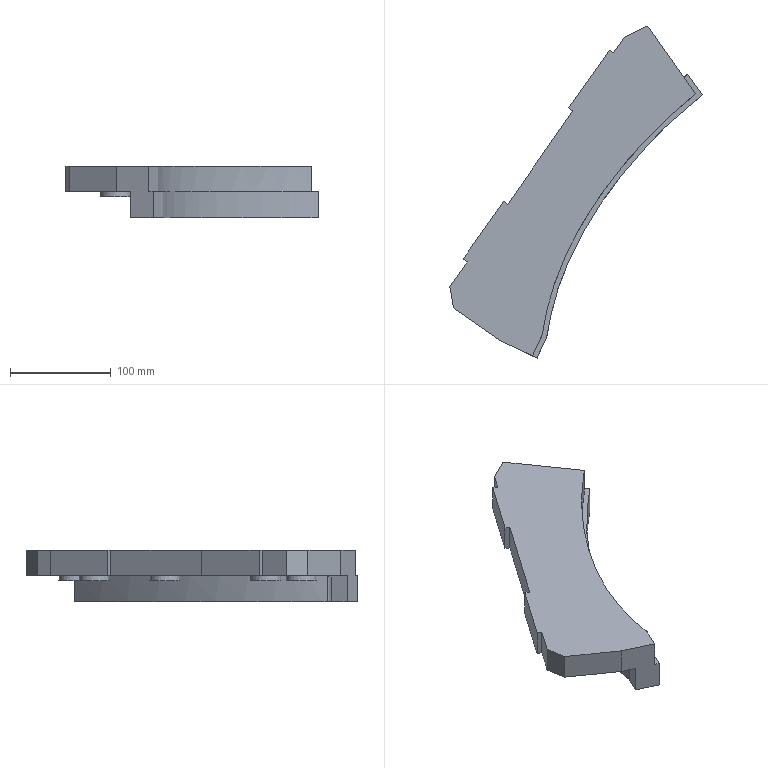Part | NX | features solid 2 | 1 solid | 32 faces | box 249.989 x 328.717 x 51 mm | volume 896333 mm3 | plane 24 | cylinder 5 | spline 3 | commonest cylinder face diameters 30 x5
STEP:
#1=CARTESIAN_POINT('',(-648.758,403.076,20.));
#2=VERTEX_POINT('',#1);
#3=CARTESIAN_POINT('',(-648.758,403.076,45.));
#4=VERTEX_POINT('',#3);
#5=CARTESIAN_POINT('',(-648.758,403.076,70.));
#6=DIRECTION('',(0.,0.,1.));
#7=VECTOR('',#6,1000.);
#8=LINE('',#5,#7);
#9=EDGE_CURVE('',#2,#4,#8,.T.);
#10=ORIENTED_EDGE('',*,*,#9,.F.);
#11=CARTESIAN_POINT('',(-672.097,391.693,20.));
#12=VERTEX_POINT('',#11);
#13=CARTESIAN_POINT('',(-659.778,397.701,20.));
#14=DIRECTION('',(-0.8988,-0.4384,0.));
#15=VECTOR('',#14,1000.);
#16=LINE('',#13,#15);
#17=EDGE_CURVE('',#12,#2,#16,.F.);
#18=ORIENTED_EDGE('',*,*,#17,.F.);
#19=CARTESIAN_POINT('',(-672.097,391.693,45.));
#20=VERTEX_POINT('',#19);
#21=CARTESIAN_POINT('',(-672.097,391.693,70.));
#22=DIRECTION('',(0.,0.,1.));
#23=VECTOR('',#22,1000.);
#24=LINE('',#21,#23);
#25=EDGE_CURVE('',#12,#20,#24,.T.);
#26=ORIENTED_EDGE('',*,*,#25,.T.);
#27=CARTESIAN_POINT('',(-659.778,397.701,45.));
#28=DIRECTION('',(0.8988,0.4384,0.));
#29=VECTOR('',#28,1000.);
#30=LINE('',#27,#29);
#31=EDGE_CURVE('',#20,#4,#30,.T.);
#32=ORIENTED_EDGE('',*,*,#31,.T.);
#33=EDGE_LOOP('',(#10,#18,#26,#32));
#34=FACE_BOUND('',#33,.T.);
#35=CARTESIAN_POINT('',(-659.778,397.701,70.));
#36=DIRECTION('',(-0.4384,0.8988,0.));
#37=DIRECTION('',(-0.8988,-0.4384,0.));
#38=AXIS2_PLACEMENT_3D('',#35,#36,#37);
#39=PLANE('',#38);
#40=ADVANCED_FACE('',(#34),#39,.T.);
#41=CARTESIAN_POINT('',(-758.462,74.359,20.));
#42=VERTEX_POINT('',#41);
#43=CARTESIAN_POINT('',(-595.,335.019,20.));
#44=VERTEX_POINT('',#43);
#45=CARTESIAN_POINT('',(-595.,335.019,20.));
#46=CARTESIAN_POINT('',(-605.153,326.905,20.));
#47=CARTESIAN_POINT('',(-620.012,314.117,20.));
#48=CARTESIAN_POINT('',(-638.944,295.82,20.));
#49=CARTESIAN_POINT('',(-657.041,276.924,20.));
#50=CARTESIAN_POINT('',(-678.202,252.077,20.));
#51=CARTESIAN_POINT('',(-697.186,225.493,20.));
#52=CARTESIAN_POINT('',(-710.926,202.978,20.));
#53=CARTESIAN_POINT('',(-720.284,185.624,20.));
#54=CARTESIAN_POINT('',(-728.613,167.785,20.));
#55=CARTESIAN_POINT('',(-735.843,149.369,20.));
#56=CARTESIAN_POINT('',(-740.793,133.659,20.));
#57=CARTESIAN_POINT('',(-744.038,120.871,20.));
#58=CARTESIAN_POINT('',(-745.744,112.807,20.));
#59=CARTESIAN_POINT('',(-746.914,106.319,20.));
#60=CARTESIAN_POINT('',(-747.543,102.244,20.));
#61=CARTESIAN_POINT('',(-748.031,98.98,20.));
#62=CARTESIAN_POINT('',(-748.271,96.487,20.));
#63=CARTESIAN_POINT('',(-749.155,94.226,20.));
#64=CARTESIAN_POINT('',(-750.586,91.301,20.));
#65=CARTESIAN_POINT('',(-752.275,87.61,20.));
#66=CARTESIAN_POINT('',(-755.033,81.723,20.));
#67=CARTESIAN_POINT('',(-757.089,77.304,20.));
#68=CARTESIAN_POINT('',(-758.462,74.359,20.));
#69=B_SPLINE_CURVE_WITH_KNOTS('',3,(#45,#46,#47,#48,#49,#50,#51,#52,#53,#54,#55,#56,#57,#58,#59,#60,#61,#62,#63,#64,#65,#66,#67,#68),.UNSPECIFIED.,.F.,.F.,(4,1,1,1,1,1,1,1,1,1,1,1,1,1,1,1,1,1,1,1,1,4),(1.053,1.092,1.112,1.131,1.17,1.209,1.228,1.248,1.267,1.287,1.306,1.316,1.326,1.33,1.335,1.338,1.34,1.343,1.345,1.35,1.355,1.364),.UNSPECIFIED.);
#70=EDGE_CURVE('',#42,#44,#69,.F.);
#71=ORIENTED_EDGE('',*,*,#70,.T.);
#72=CARTESIAN_POINT('',(-609.367,355.537,20.));
#73=VERTEX_POINT('',#72);
#74=CARTESIAN_POINT('',(-595.62,335.904,20.));
#75=DIRECTION('',(-0.5736,0.8192,0.));
#76=VECTOR('',#75,1000.);
#77=LINE('',#74,#76);
#78=EDGE_CURVE('',#73,#44,#77,.F.);
#79=ORIENTED_EDGE('',*,*,#78,.F.);
#80=CARTESIAN_POINT('',(-613.276,352.402,20.));
#81=VERTEX_POINT('',#80);
#82=CARTESIAN_POINT('',(-613.276,352.402,20.));
#83=CARTESIAN_POINT('',(-611.977,353.453,20.));
#84=CARTESIAN_POINT('',(-610.674,354.498,20.));
#85=CARTESIAN_POINT('',(-609.367,355.537,20.));
#86=B_SPLINE_CURVE_WITH_KNOTS('',3,(#82,#83,#84,#85),.UNSPECIFIED.,.F.,.F.,(4,4),(0.8753,0.8887),.UNSPECIFIED.);
#87=EDGE_CURVE('',#81,#73,#86,.T.);
#88=ORIENTED_EDGE('',*,*,#87,.F.);
#89=CARTESIAN_POINT('',(-601.776,335.978,20.));
#90=VERTEX_POINT('',#89);
#91=CARTESIAN_POINT('',(-601.969,336.255,20.));
#92=DIRECTION('',(0.5736,-0.8192,0.));
#93=VECTOR('',#92,1000.);
#94=LINE('',#91,#93);
#95=EDGE_CURVE('',#90,#81,#94,.F.);
#96=ORIENTED_EDGE('',*,*,#95,.F.);
#97=CARTESIAN_POINT('',(-762.994,76.472,20.));
#98=VERTEX_POINT('',#97);
#99=CARTESIAN_POINT('',(-601.776,335.978,20.));
#100=CARTESIAN_POINT('',(-611.865,327.771,20.));
#101=CARTESIAN_POINT('',(-631.456,310.599,20.));
#102=CARTESIAN_POINT('',(-658.632,282.914,20.));
#103=CARTESIAN_POINT('',(-683.631,253.231,20.));
#104=CARTESIAN_POINT('',(-702.468,226.555,20.));
#105=CARTESIAN_POINT('',(-715.855,204.414,20.));
#106=CARTESIAN_POINT('',(-725.004,187.347,20.));
#107=CARTESIAN_POINT('',(-733.184,169.786,20.));
#108=CARTESIAN_POINT('',(-740.313,151.694,20.));
#109=CARTESIAN_POINT('',(-745.285,136.104,20.));
#110=CARTESIAN_POINT('',(-748.577,123.395,20.));
#111=CARTESIAN_POINT('',(-750.336,115.344,20.));
#112=CARTESIAN_POINT('',(-751.55,108.834,20.));
#113=CARTESIAN_POINT('',(-752.231,104.739,20.));
#114=CARTESIAN_POINT('',(-752.713,101.439,20.));
#115=CARTESIAN_POINT('',(-753.022,99.38,20.));
#116=CARTESIAN_POINT('',(-753.186,97.703,20.));
#117=CARTESIAN_POINT('',(-753.603,96.55,20.));
#118=CARTESIAN_POINT('',(-754.149,95.443,20.));
#119=CARTESIAN_POINT('',(-754.839,93.954,20.));
#120=CARTESIAN_POINT('',(-755.709,92.095,20.));
#121=CARTESIAN_POINT('',(-757.096,89.119,20.));
#122=CARTESIAN_POINT('',(-758.831,85.399,20.));
#123=CARTESIAN_POINT('',(-760.912,80.936,20.));
#124=CARTESIAN_POINT('',(-762.3,77.96,20.));
#125=CARTESIAN_POINT('',(-762.994,76.472,20.));
#126=B_SPLINE_CURVE_WITH_KNOTS('',3,(#99,#100,#101,#102,#103,#104,#105,#106,#107,#108,#109,#110,#111,#112,#113,#114,#115,#116,#117,#118,#119,#120,#121,#122,#123,#124,#125),.UNSPECIFIED.,.F.,.F.,(4,1,1,1,1,1,1,1,1,1,1,1,1,1,1,1,1,1,1,1,1,1,1,1,4),(0.8327,0.8717,0.9106,0.9496,0.9886,1.008,1.028,1.047,1.066,1.086,1.096,1.105,1.11,1.115,1.118,1.12,1.121,1.122,1.124,1.125,1.127,1.13,1.135,1.14,1.144),.UNSPECIFIED.);
#127=EDGE_CURVE('',#98,#90,#126,.F.);
#128=ORIENTED_EDGE('',*,*,#127,.F.);
#129=CARTESIAN_POINT('',(-758.462,74.359,20.));
#130=DIRECTION('',(-0.9063,0.4226,0.));
#131=VECTOR('',#130,1000.);
#132=LINE('',#129,#131);
#133=EDGE_CURVE('',#98,#42,#132,.F.);
#134=ORIENTED_EDGE('',*,*,#133,.T.);
#135=EDGE_LOOP('',(#71,#79,#88,#96,#128,#134));
#136=FACE_BOUND('',#135,.T.);
#137=CARTESIAN_POINT('',(-561.977,359.461,20.));
#138=DIRECTION('',(0.,0.,1.));
#139=DIRECTION('',(1.,0.,0.));
#140=AXIS2_PLACEMENT_3D('',#137,#138,#139);
#141=PLANE('',#140);
#142=ADVANCED_FACE('',(#136),#141,.T.);
#143=CARTESIAN_POINT('',(-595.,335.019,-6.));
#144=VERTEX_POINT('',#143);
#145=CARTESIAN_POINT('',(-595.,335.019,7.));
#146=DIRECTION('',(0.,0.,-1.));
#147=VECTOR('',#146,1000.);
#148=LINE('',#145,#147);
#149=EDGE_CURVE('',#44,#144,#148,.T.);
#150=ORIENTED_EDGE('',*,*,#149,.F.);
#151=ORIENTED_EDGE('',*,*,#70,.F.);
#152=CARTESIAN_POINT('',(-758.462,74.359,-6.));
#153=VERTEX_POINT('',#152);
#154=CARTESIAN_POINT('',(-758.462,74.359,70.));
#155=DIRECTION('',(0.,0.,-1.));
#156=VECTOR('',#155,1000.);
#157=LINE('',#154,#156);
#158=EDGE_CURVE('',#42,#153,#157,.T.);
#159=ORIENTED_EDGE('',*,*,#158,.T.);
#160=CARTESIAN_POINT('',(-595.,335.019,-6.));
#161=CARTESIAN_POINT('',(-605.196,326.871,-6.));
#162=CARTESIAN_POINT('',(-625.159,309.672,-6.));
#163=CARTESIAN_POINT('',(-652.791,281.906,-6.));
#164=CARTESIAN_POINT('',(-678.136,252.163,-6.));
#165=CARTESIAN_POINT('',(-697.173,225.515,-6.));
#166=CARTESIAN_POINT('',(-710.901,203.021,-6.));
#167=CARTESIAN_POINT('',(-720.24,185.709,-6.));
#168=CARTESIAN_POINT('',(-728.575,167.875,-6.));
#169=CARTESIAN_POINT('',(-735.812,149.456,-6.));
#170=CARTESIAN_POINT('',(-740.761,133.769,-6.));
#171=CARTESIAN_POINT('',(-744.012,120.984,-6.));
#172=CARTESIAN_POINT('',(-745.72,112.928,-6.));
#173=CARTESIAN_POINT('',(-746.895,106.436,-6.));
#174=CARTESIAN_POINT('',(-747.528,102.339,-6.));
#175=CARTESIAN_POINT('',(-748.022,99.056,-6.));
#176=CARTESIAN_POINT('',(-748.26,96.545,-6.));
#177=CARTESIAN_POINT('',(-749.131,94.27,-6.));
#178=CARTESIAN_POINT('',(-750.569,91.341,-6.));
#179=CARTESIAN_POINT('',(-752.26,87.64,-6.));
#180=CARTESIAN_POINT('',(-754.334,83.216,-6.));
#181=CARTESIAN_POINT('',(-756.397,78.787,-6.));
#182=CARTESIAN_POINT('',(-757.774,75.835,-6.));
#183=CARTESIAN_POINT('',(-758.462,74.359,-6.));
#184=B_SPLINE_CURVE_WITH_KNOTS('',3,(#160,#161,#162,#163,#164,#165,#166,#167,#168,#169,#170,#171,#172,#173,#174,#175,#176,#177,#178,#179,#180,#181,#182,#183),.UNSPECIFIED.,.F.,.F.,(4,1,1,1,1,1,1,1,1,1,1,1,1,1,1,1,1,1,1,1,1,4),(1.071,1.11,1.149,1.188,1.227,1.246,1.266,1.285,1.305,1.324,1.334,1.344,1.348,1.353,1.356,1.358,1.361,1.363,1.368,1.373,1.378,1.382),.UNSPECIFIED.);
#185=EDGE_CURVE('',#153,#144,#184,.F.);
#186=ORIENTED_EDGE('',*,*,#185,.T.);
#187=EDGE_LOOP('',(#150,#151,#159,#186));
#188=FACE_BOUND('',#187,.T.);
#189=CARTESIAN_POINT('',(-758.462,74.359,20.));
#190=CARTESIAN_POINT('',(-758.462,74.359,-6.));
#191=CARTESIAN_POINT('',(-757.77,75.844,20.));
#192=CARTESIAN_POINT('',(-757.77,75.844,-6.));
#193=CARTESIAN_POINT('',(-756.384,78.814,20.));
#194=CARTESIAN_POINT('',(-756.384,78.814,-6.));
#195=CARTESIAN_POINT('',(-754.31,83.27,20.));
#196=CARTESIAN_POINT('',(-754.31,83.27,-6.));
#197=CARTESIAN_POINT('',(-752.221,87.72,20.));
#198=CARTESIAN_POINT('',(-752.221,87.72,-6.));
#199=CARTESIAN_POINT('',(-750.525,91.449,20.));
#200=CARTESIAN_POINT('',(-750.525,91.449,-6.));
#201=CARTESIAN_POINT('',(-749.067,94.385,20.));
#202=CARTESIAN_POINT('',(-749.067,94.385,-6.));
#203=CARTESIAN_POINT('',(-748.233,96.708,20.));
#204=CARTESIAN_POINT('',(-748.233,96.708,-6.));
#205=CARTESIAN_POINT('',(-748.008,99.169,20.));
#206=CARTESIAN_POINT('',(-748.008,99.169,-6.));
#207=CARTESIAN_POINT('',(-747.517,102.405,20.));
#208=CARTESIAN_POINT('',(-747.517,102.405,-6.));
#209=CARTESIAN_POINT('',(-746.892,106.453,20.));
#210=CARTESIAN_POINT('',(-746.892,106.453,-6.));
#211=CARTESIAN_POINT('',(-745.725,112.898,20.));
#212=CARTESIAN_POINT('',(-745.725,112.898,-6.));
#213=CARTESIAN_POINT('',(-744.029,120.909,20.));
#214=CARTESIAN_POINT('',(-744.029,120.909,-6.));
#215=CARTESIAN_POINT('',(-740.804,133.612,20.));
#216=CARTESIAN_POINT('',(-740.804,133.612,-6.));
#217=CARTESIAN_POINT('',(-735.88,149.258,20.));
#218=CARTESIAN_POINT('',(-735.88,149.258,-6.));
#219=CARTESIAN_POINT('',(-728.697,167.587,20.));
#220=CARTESIAN_POINT('',(-728.697,167.587,-6.));
#221=CARTESIAN_POINT('',(-720.391,185.411,20.));
#222=CARTESIAN_POINT('',(-720.391,185.411,-6.));
#223=CARTESIAN_POINT('',(-711.068,202.728,20.));
#224=CARTESIAN_POINT('',(-711.068,202.728,-6.));
#225=CARTESIAN_POINT('',(-697.423,225.135,20.));
#226=CARTESIAN_POINT('',(-697.423,225.135,-6.));
#227=CARTESIAN_POINT('',(-678.389,251.849,20.));
#228=CARTESIAN_POINT('',(-678.389,251.849,-6.));
#229=CARTESIAN_POINT('',(-644.374,291.818,20.));
#230=CARTESIAN_POINT('',(-644.374,291.818,-6.));
#231=CARTESIAN_POINT('',(-615.478,318.655,20.));
#232=CARTESIAN_POINT('',(-615.478,318.655,-6.));
#233=CARTESIAN_POINT('',(-595.,335.019,20.));
#234=CARTESIAN_POINT('',(-595.,335.019,-6.));
#235=B_SPLINE_SURFACE_WITH_KNOTS('',3,1,((#189,#190),(#191,#192),(#193,#194),(#195,#196),(#197,#198),(#199,#200),(#201,#202),(#203,#204),(#205,#206),(#207,#208),(#209,#210),(#211,#212),(#213,#214),(#215,#216),(#217,#218),(#219,#220),(#221,#222),(#223,#224),(#225,#226),(#227,#228),(#229,#230),(#231,#232),(#233,#234)),.SURF_OF_LINEAR_EXTRUSION.,.F.,.F.,.F.,(4,1,1,1,1,1,1,1,1,1,1,1,1,1,1,1,1,1,1,1,4),(2,2),(0.003106,0.007303,0.0115,0.01569,0.01989,0.02199,0.02409,0.02619,0.02828,0.03248,0.03668,0.04507,0.05346,0.07025,0.08703,0.1038,0.1206,0.1374,0.171,0.2045,0.2717),(0.,1.),.UNSPECIFIED.);
#236=ADVANCED_FACE('',(#188),#235,.F.);
#237=CARTESIAN_POINT('',(-609.367,355.537,-6.));
#238=VERTEX_POINT('',#237);
#239=CARTESIAN_POINT('',(105.312,-665.13,-6.));
#240=DIRECTION('',(-0.5736,0.8192,0.));
#241=VECTOR('',#240,1000.);
#242=LINE('',#239,#241);
#243=EDGE_CURVE('',#144,#238,#242,.T.);
#244=ORIENTED_EDGE('',*,*,#243,.F.);
#245=ORIENTED_EDGE('',*,*,#185,.F.);
#246=CARTESIAN_POINT('',(-781.12,84.924,-6.));
#247=VERTEX_POINT('',#246);
#248=CARTESIAN_POINT('',(-2805.507,1028.912,-6.));
#249=DIRECTION('',(0.9063,-0.4226,0.));
#250=VECTOR('',#249,1000.);
#251=LINE('',#248,#250);
#252=EDGE_CURVE('',#247,#153,#251,.T.);
#253=ORIENTED_EDGE('',*,*,#252,.F.);
#254=CARTESIAN_POINT('',(-609.367,355.537,-6.));
#255=CARTESIAN_POINT('',(-630.504,338.743,-6.));
#256=CARTESIAN_POINT('',(-670.028,302.396,-6.));
#257=CARTESIAN_POINT('',(-712.936,248.72,-6.));
#258=CARTESIAN_POINT('',(-740.771,201.703,-6.));
#259=CARTESIAN_POINT('',(-754.778,170.697,-6.));
#260=CARTESIAN_POINT('',(-763.749,144.683,-6.));
#261=CARTESIAN_POINT('',(-768.036,127.873,-6.));
#262=CARTESIAN_POINT('',(-771.159,114.324,-6.));
#263=CARTESIAN_POINT('',(-771.858,103.55,-6.));
#264=CARTESIAN_POINT('',(-776.875,94.381,-6.));
#265=CARTESIAN_POINT('',(-779.658,88.059,-6.));
#266=CARTESIAN_POINT('',(-781.12,84.924,-6.));
#267=B_SPLINE_CURVE_WITH_KNOTS('',3,(#254,#255,#256,#257,#258,#259,#260,#261,#262,#263,#264,#265,#266),.UNSPECIFIED.,.F.,.F.,(4,1,1,1,1,1,1,1,1,1,4),(0.205,0.2866,0.3682,0.409,0.4498,0.4702,0.4906,0.5008,0.511,0.5212,0.5314),.UNSPECIFIED.);
#268=EDGE_CURVE('',#247,#238,#267,.F.);
#269=ORIENTED_EDGE('',*,*,#268,.T.);
#270=EDGE_LOOP('',(#244,#245,#253,#269));
#271=FACE_BOUND('',#270,.T.);
#272=CARTESIAN_POINT('',(-80.139,-794.984,-6.));
#273=DIRECTION('',(0.,0.,1.));
#274=DIRECTION('',(1.,0.,0.));
#275=AXIS2_PLACEMENT_3D('',#272,#273,#274);
#276=PLANE('',#275);
#277=ADVANCED_FACE('',(#271),#276,.F.);
#278=CARTESIAN_POINT('',(-601.776,335.978,45.));
#279=VERTEX_POINT('',#278);
#280=CARTESIAN_POINT('',(-601.969,336.255,45.));
#281=DIRECTION('',(-0.5736,0.8192,0.));
#282=VECTOR('',#281,1000.);
#283=LINE('',#280,#282);
#284=EDGE_CURVE('',#279,#4,#283,.T.);
#285=ORIENTED_EDGE('',*,*,#284,.T.);
#286=ORIENTED_EDGE('',*,*,#31,.F.);
#287=CARTESIAN_POINT('',(-682.817,376.384,45.));
#288=VERTEX_POINT('',#287);
#289=CARTESIAN_POINT('',(-902.294,62.938,45.));
#290=DIRECTION('',(0.5736,0.8192,0.));
#291=VECTOR('',#290,1000.);
#292=LINE('',#289,#291);
#293=EDGE_CURVE('',#288,#20,#292,.T.);
#294=ORIENTED_EDGE('',*,*,#293,.F.);
#295=CARTESIAN_POINT('',(-686.912,379.252,45.));
#296=VERTEX_POINT('',#295);
#297=CARTESIAN_POINT('',(271.949,-292.15,45.));
#298=DIRECTION('',(-0.8192,0.5736,0.));
#299=VECTOR('',#298,1000.);
#300=LINE('',#297,#299);
#301=EDGE_CURVE('',#288,#296,#300,.T.);
#302=ORIENTED_EDGE('',*,*,#301,.T.);
#303=CARTESIAN_POINT('',(-727.063,321.911,45.));
#304=VERTEX_POINT('',#303);
#305=CARTESIAN_POINT('',(-675.441,395.635,45.));
#306=DIRECTION('',(0.5736,0.8192,0.));
#307=VECTOR('',#306,1000.);
#308=LINE('',#305,#307);
#309=EDGE_CURVE('',#304,#296,#308,.T.);
#310=ORIENTED_EDGE('',*,*,#309,.F.);
#311=CARTESIAN_POINT('',(-722.967,319.043,45.));
#312=VERTEX_POINT('',#311);
#313=CARTESIAN_POINT('',(231.799,-349.491,45.));
#314=DIRECTION('',(-0.8192,0.5736,0.));
#315=VECTOR('',#314,1000.);
#316=LINE('',#313,#315);
#317=EDGE_CURVE('',#312,#304,#316,.T.);
#318=ORIENTED_EDGE('',*,*,#317,.F.);
#319=CARTESIAN_POINT('',(-787.631,226.693,45.));
#320=VERTEX_POINT('',#319);
#321=CARTESIAN_POINT('',(-902.294,62.938,45.));
#322=DIRECTION('',(0.5736,0.8192,0.));
#323=VECTOR('',#322,1000.);
#324=LINE('',#321,#323);
#325=EDGE_CURVE('',#320,#312,#324,.T.);
#326=ORIENTED_EDGE('',*,*,#325,.F.);
#327=CARTESIAN_POINT('',(-791.727,229.561,45.));
#328=VERTEX_POINT('',#327);
#329=CARTESIAN_POINT('',(167.134,-441.841,45.));
#330=DIRECTION('',(-0.8192,0.5736,0.));
#331=VECTOR('',#330,1000.);
#332=LINE('',#329,#331);
#333=EDGE_CURVE('',#320,#328,#332,.T.);
#334=ORIENTED_EDGE('',*,*,#333,.T.);
#335=CARTESIAN_POINT('',(-831.877,172.22,45.));
#336=VERTEX_POINT('',#335);
#337=CARTESIAN_POINT('',(-846.217,151.741,45.));
#338=DIRECTION('',(0.5736,0.8192,0.));
#339=VECTOR('',#338,1000.);
#340=LINE('',#337,#339);
#341=EDGE_CURVE('',#336,#328,#340,.T.);
#342=ORIENTED_EDGE('',*,*,#341,.F.);
#343=CARTESIAN_POINT('',(-827.782,169.352,45.));
#344=VERTEX_POINT('',#343);
#345=CARTESIAN_POINT('',(126.984,-499.182,45.));
#346=DIRECTION('',(-0.8192,0.5736,0.));
#347=VECTOR('',#346,1000.);
#348=LINE('',#345,#347);
#349=EDGE_CURVE('',#344,#336,#348,.T.);
#350=ORIENTED_EDGE('',*,*,#349,.F.);
#351=CARTESIAN_POINT('',(-844.989,144.778,45.));
#352=VERTEX_POINT('',#351);
#353=CARTESIAN_POINT('',(-902.294,62.938,45.));
#354=DIRECTION('',(0.5736,0.8192,0.));
#355=VECTOR('',#354,1000.);
#356=LINE('',#353,#355);
#357=EDGE_CURVE('',#352,#344,#356,.T.);
#358=ORIENTED_EDGE('',*,*,#357,.F.);
#359=CARTESIAN_POINT('',(-841.305,123.887,45.));
#360=VERTEX_POINT('',#359);
#361=CARTESIAN_POINT('',(-799.958,-110.607,45.));
#362=DIRECTION('',(-0.1736,0.9848,0.));
#363=VECTOR('',#362,1000.);
#364=LINE('',#361,#363);
#365=EDGE_CURVE('',#352,#360,#364,.F.);
#366=ORIENTED_EDGE('',*,*,#365,.T.);
#367=CARTESIAN_POINT('',(-794.714,91.264,45.));
#368=VERTEX_POINT('',#367);
#369=CARTESIAN_POINT('',(-875.296,147.687,45.));
#370=DIRECTION('',(-0.8192,0.5736,0.));
#371=VECTOR('',#370,1000.);
#372=LINE('',#369,#371);
#373=EDGE_CURVE('',#360,#368,#372,.F.);
#374=ORIENTED_EDGE('',*,*,#373,.T.);
#375=CARTESIAN_POINT('',(-762.994,76.472,45.));
#376=VERTEX_POINT('',#375);
#377=CARTESIAN_POINT('',(-2805.507,1028.912,45.));
#378=DIRECTION('',(0.9063,-0.4226,0.));
#379=VECTOR('',#378,1000.);
#380=LINE('',#377,#379);
#381=EDGE_CURVE('',#368,#376,#380,.T.);
#382=ORIENTED_EDGE('',*,*,#381,.T.);
#383=CARTESIAN_POINT('',(-762.994,76.472,45.));
#384=CARTESIAN_POINT('',(-762.296,77.969,45.));
#385=CARTESIAN_POINT('',(-760.899,80.963,45.));
#386=CARTESIAN_POINT('',(-758.805,85.454,45.));
#387=CARTESIAN_POINT('',(-757.06,89.196,45.));
#388=CARTESIAN_POINT('',(-755.665,92.19,45.));
#389=CARTESIAN_POINT('',(-754.789,94.061,45.));
#390=CARTESIAN_POINT('',(-754.096,95.559,45.));
#391=CARTESIAN_POINT('',(-753.541,96.672,45.));
#392=CARTESIAN_POINT('',(-753.168,97.842,45.));
#393=CARTESIAN_POINT('',(-753.006,99.505,45.));
#394=CARTESIAN_POINT('',(-752.696,101.551,45.));
#395=CARTESIAN_POINT('',(-752.217,104.829,45.));
#396=CARTESIAN_POINT('',(-751.537,108.902,45.));
#397=CARTESIAN_POINT('',(-750.329,115.381,45.));
#398=CARTESIAN_POINT('',(-748.574,123.409,45.));
#399=CARTESIAN_POINT('',(-745.293,136.072,45.));
#400=CARTESIAN_POINT('',(-740.361,151.552,45.));
#401=CARTESIAN_POINT('',(-733.25,169.635,45.));
#402=CARTESIAN_POINT('',(-725.048,187.263,45.));
#403=CARTESIAN_POINT('',(-715.826,204.474,45.));
#404=CARTESIAN_POINT('',(-702.266,226.868,45.));
#405=CARTESIAN_POINT('',(-683.587,253.27,45.));
#406=CARTESIAN_POINT('',(-658.666,282.876,45.));
#407=CARTESIAN_POINT('',(-631.52,310.539,45.));
#408=CARTESIAN_POINT('',(-611.886,327.754,45.));
#409=CARTESIAN_POINT('',(-601.776,335.978,45.));
#410=B_SPLINE_CURVE_WITH_KNOTS('',3,(#383,#384,#385,#386,#387,#388,#389,#390,#391,#392,#393,#394,#395,#396,#397,#398,#399,#400,#401,#402,#403,#404,#405,#406,#407,#408,#409),.UNSPECIFIED.,.F.,.F.,(4,1,1,1,1,1,1,1,1,1,1,1,1,1,1,1,1,1,1,1,1,1,1,1,4),(0.,0.00491,0.00982,0.01473,0.01718,0.01964,0.02087,0.02209,0.02332,0.02455,0.027,0.02946,0.03437,0.03928,0.0491,0.05892,0.07856,0.0982,0.1178,0.1375,0.1571,0.1964,0.2357,0.2749,0.3142),.UNSPECIFIED.);
#411=EDGE_CURVE('',#376,#279,#410,.T.);
#412=ORIENTED_EDGE('',*,*,#411,.T.);
#413=EDGE_LOOP('',(#285,#286,#294,#302,#310,#318,#326,#334,#342,#350,#358,#366,#374,#382,#412));
#414=FACE_BOUND('',#413,.T.);
#415=CARTESIAN_POINT('',(-80.139,-794.984,45.));
#416=DIRECTION('',(0.,0.,1.));
#417=DIRECTION('',(1.,0.,0.));
#418=AXIS2_PLACEMENT_3D('',#415,#416,#417);
#419=PLANE('',#418);
#420=ADVANCED_FACE('',(#414),#419,.T.);
#421=CARTESIAN_POINT('',(-660.611,355.558,20.));
#422=VERTEX_POINT('',#421);
#423=CARTESIAN_POINT('',(-645.611,355.558,20.));
#424=DIRECTION('',(0.,0.,-1.));
#425=DIRECTION('',(-1.,0.,0.));
#426=AXIS2_PLACEMENT_3D('',#423,#424,#425);
#427=CIRCLE('',#426,15.);
#428=EDGE_CURVE('',#422,#422,#427,.F.);
#429=ORIENTED_EDGE('',*,*,#428,.T.);
#430=EDGE_LOOP('',(#429));
#431=FACE_BOUND('',#430,.T.);
#432=CARTESIAN_POINT('',(-690.611,335.558,20.));
#433=VERTEX_POINT('',#432);
#434=CARTESIAN_POINT('',(-675.611,335.558,20.));
#435=DIRECTION('',(0.,0.,-1.));
#436=DIRECTION('',(-1.,0.,0.));
#437=AXIS2_PLACEMENT_3D('',#434,#435,#436);
#438=CIRCLE('',#437,15.);
#439=EDGE_CURVE('',#433,#433,#438,.F.);
#440=ORIENTED_EDGE('',*,*,#439,.T.);
#441=EDGE_LOOP('',(#440));
#442=FACE_BOUND('',#441,.T.);
#443=CARTESIAN_POINT('',(-810.611,130.558,20.));
#444=VERTEX_POINT('',#443);
#445=CARTESIAN_POINT('',(-795.611,130.558,20.));
#446=DIRECTION('',(0.,0.,-1.));
#447=DIRECTION('',(-1.,0.,0.));
#448=AXIS2_PLACEMENT_3D('',#445,#446,#447);
#449=CIRCLE('',#448,15.);
#450=EDGE_CURVE('',#444,#444,#449,.T.);
#451=ORIENTED_EDGE('',*,*,#450,.F.);
#452=EDGE_LOOP('',(#451));
#453=FACE_BOUND('',#452,.T.);
#454=CARTESIAN_POINT('',(-810.611,165.558,20.));
#455=VERTEX_POINT('',#454);
#456=CARTESIAN_POINT('',(-795.611,165.558,20.));
#457=DIRECTION('',(0.,0.,-1.));
#458=DIRECTION('',(-1.,0.,0.));
#459=AXIS2_PLACEMENT_3D('',#456,#457,#458);
#460=CIRCLE('',#459,15.);
#461=EDGE_CURVE('',#455,#455,#460,.T.);
#462=ORIENTED_EDGE('',*,*,#461,.F.);
#463=EDGE_LOOP('',(#462));
#464=FACE_BOUND('',#463,.T.);
#465=CARTESIAN_POINT('',(-735.611,265.558,20.));
#466=VERTEX_POINT('',#465);
#467=CARTESIAN_POINT('',(-720.611,265.558,20.));
#468=DIRECTION('',(0.,0.,-1.));
#469=DIRECTION('',(-1.,0.,0.));
#470=AXIS2_PLACEMENT_3D('',#467,#468,#469);
#471=CIRCLE('',#470,15.);
#472=EDGE_CURVE('',#466,#466,#471,.T.);
#473=ORIENTED_EDGE('',*,*,#472,.F.);
#474=EDGE_LOOP('',(#473));
#475=FACE_BOUND('',#474,.T.);
#476=ORIENTED_EDGE('',*,*,#17,.T.);
#477=CARTESIAN_POINT('',(-601.969,336.255,20.));
#478=DIRECTION('',(0.5736,-0.8192,0.));
#479=VECTOR('',#478,1000.);
#480=LINE('',#477,#479);
#481=EDGE_CURVE('',#81,#2,#480,.F.);
#482=ORIENTED_EDGE('',*,*,#481,.F.);
#483=CARTESIAN_POINT('',(-781.12,84.924,20.));
#484=VERTEX_POINT('',#483);
#485=CARTESIAN_POINT('',(-613.276,352.402,20.));
#486=CARTESIAN_POINT('',(-633.961,335.665,20.));
#487=CARTESIAN_POINT('',(-672.617,299.523,20.));
#488=CARTESIAN_POINT('',(-714.519,246.391,20.));
#489=CARTESIAN_POINT('',(-741.653,199.957,20.));
#490=CARTESIAN_POINT('',(-755.295,169.366,20.));
#491=CARTESIAN_POINT('',(-764.029,143.734,20.));
#492=CARTESIAN_POINT('',(-768.193,127.17,20.));
#493=CARTESIAN_POINT('',(-771.254,113.831,20.));
#494=CARTESIAN_POINT('',(-771.879,103.202,20.));
#495=CARTESIAN_POINT('',(-776.98,94.242,20.));
#496=CARTESIAN_POINT('',(-779.682,88.009,20.));
#497=CARTESIAN_POINT('',(-781.12,84.924,20.));
#498=B_SPLINE_CURVE_WITH_KNOTS('',3,(#485,#486,#487,#488,#489,#490,#491,#492,#493,#494,#495,#496,#497),.UNSPECIFIED.,.F.,.F.,(4,1,1,1,1,1,1,1,1,1,4),(0.9033,0.9838,1.064,1.105,1.145,1.165,1.185,1.195,1.205,1.215,1.225),.UNSPECIFIED.);
#499=EDGE_CURVE('',#484,#81,#498,.F.);
#500=ORIENTED_EDGE('',*,*,#499,.F.);
#501=CARTESIAN_POINT('',(-794.714,91.264,20.));
#502=VERTEX_POINT('',#501);
#503=CARTESIAN_POINT('',(-2805.507,1028.912,20.));
#504=DIRECTION('',(-0.9063,0.4226,0.));
#505=VECTOR('',#504,1000.);
#506=LINE('',#503,#505);
#507=EDGE_CURVE('',#502,#484,#506,.F.);
#508=ORIENTED_EDGE('',*,*,#507,.F.);
#509=CARTESIAN_POINT('',(-841.305,123.887,20.));
#510=VERTEX_POINT('',#509);
#511=CARTESIAN_POINT('',(-762.446,68.669,20.));
#512=DIRECTION('',(-0.8192,0.5736,0.));
#513=VECTOR('',#512,1000.);
#514=LINE('',#511,#513);
#515=EDGE_CURVE('',#502,#510,#514,.T.);
#516=ORIENTED_EDGE('',*,*,#515,.T.);
#517=CARTESIAN_POINT('',(-844.989,144.778,20.));
#518=VERTEX_POINT('',#517);
#519=CARTESIAN_POINT('',(-841.305,123.887,20.));
#520=DIRECTION('',(-0.1736,0.9848,0.));
#521=VECTOR('',#520,1000.);
#522=LINE('',#519,#521);
#523=EDGE_CURVE('',#510,#518,#522,.T.);
#524=ORIENTED_EDGE('',*,*,#523,.T.);
#525=CARTESIAN_POINT('',(-827.782,169.352,20.));
#526=VERTEX_POINT('',#525);
#527=CARTESIAN_POINT('',(-902.294,62.938,20.));
#528=DIRECTION('',(-0.5736,-0.8192,0.));
#529=VECTOR('',#528,1000.);
#530=LINE('',#527,#529);
#531=EDGE_CURVE('',#518,#526,#530,.F.);
#532=ORIENTED_EDGE('',*,*,#531,.T.);
#533=CARTESIAN_POINT('',(-831.877,172.22,20.));
#534=VERTEX_POINT('',#533);
#535=CARTESIAN_POINT('',(-738.746,107.009,20.));
#536=DIRECTION('',(0.8192,-0.5736,0.));
#537=VECTOR('',#536,1000.);
#538=LINE('',#535,#537);
#539=EDGE_CURVE('',#526,#534,#538,.F.);
#540=ORIENTED_EDGE('',*,*,#539,.T.);
#541=CARTESIAN_POINT('',(-791.727,229.561,20.));
#542=VERTEX_POINT('',#541);
#543=CARTESIAN_POINT('',(-846.217,151.741,20.));
#544=DIRECTION('',(0.5736,0.8192,0.));
#545=VECTOR('',#544,1000.);
#546=LINE('',#543,#545);
#547=EDGE_CURVE('',#534,#542,#546,.T.);
#548=ORIENTED_EDGE('',*,*,#547,.T.);
#549=CARTESIAN_POINT('',(-787.631,226.693,20.));
#550=VERTEX_POINT('',#549);
#551=CARTESIAN_POINT('',(-698.596,164.349,20.));
#552=DIRECTION('',(0.8192,-0.5736,0.));
#553=VECTOR('',#552,1000.);
#554=LINE('',#551,#553);
#555=EDGE_CURVE('',#550,#542,#554,.F.);
#556=ORIENTED_EDGE('',*,*,#555,.F.);
#557=CARTESIAN_POINT('',(-722.967,319.043,20.));
#558=VERTEX_POINT('',#557);
#559=CARTESIAN_POINT('',(-902.294,62.938,20.));
#560=DIRECTION('',(-0.5736,-0.8192,0.));
#561=VECTOR('',#560,1000.);
#562=LINE('',#559,#561);
#563=EDGE_CURVE('',#550,#558,#562,.F.);
#564=ORIENTED_EDGE('',*,*,#563,.T.);
#565=CARTESIAN_POINT('',(-727.063,321.911,20.));
#566=VERTEX_POINT('',#565);
#567=CARTESIAN_POINT('',(-633.931,256.7,20.));
#568=DIRECTION('',(0.8192,-0.5736,0.));
#569=VECTOR('',#568,1000.);
#570=LINE('',#567,#569);
#571=EDGE_CURVE('',#558,#566,#570,.F.);
#572=ORIENTED_EDGE('',*,*,#571,.T.);
#573=CARTESIAN_POINT('',(-686.912,379.252,20.));
#574=VERTEX_POINT('',#573);
#575=CARTESIAN_POINT('',(-675.441,395.635,20.));
#576=DIRECTION('',(0.5736,0.8192,0.));
#577=VECTOR('',#576,1000.);
#578=LINE('',#575,#577);
#579=EDGE_CURVE('',#566,#574,#578,.T.);
#580=ORIENTED_EDGE('',*,*,#579,.T.);
#581=CARTESIAN_POINT('',(-682.817,376.384,20.));
#582=VERTEX_POINT('',#581);
#583=CARTESIAN_POINT('',(-593.781,314.04,20.));
#584=DIRECTION('',(0.8192,-0.5736,0.));
#585=VECTOR('',#584,1000.);
#586=LINE('',#583,#585);
#587=EDGE_CURVE('',#582,#574,#586,.F.);
#588=ORIENTED_EDGE('',*,*,#587,.F.);
#589=CARTESIAN_POINT('',(-902.294,62.938,20.));
#590=DIRECTION('',(-0.5736,-0.8192,0.));
#591=VECTOR('',#590,1000.);
#592=LINE('',#589,#591);
#593=EDGE_CURVE('',#582,#12,#592,.F.);
#594=ORIENTED_EDGE('',*,*,#593,.T.);
#595=EDGE_LOOP('',(#476,#482,#500,#508,#516,#524,#532,#540,#548,#556,#564,#572,#580,#588,#594));
#596=FACE_BOUND('',#595,.T.);
#597=CARTESIAN_POINT('',(-561.977,359.461,20.));
#598=DIRECTION('',(0.,0.,-1.));
#599=DIRECTION('',(-1.,0.,0.));
#600=AXIS2_PLACEMENT_3D('',#597,#598,#599);
#601=PLANE('',#600);
#602=ADVANCED_FACE('',(#431,#442,#453,#464,#475,#596),#601,.T.);
#603=CARTESIAN_POINT('',(-609.367,355.537,7.));
#604=DIRECTION('',(0.,0.,1.));
#605=VECTOR('',#604,1000.);
#606=LINE('',#603,#605);
#607=EDGE_CURVE('',#238,#73,#606,.T.);
#608=ORIENTED_EDGE('',*,*,#607,.F.);
#609=ORIENTED_EDGE('',*,*,#268,.F.);
#610=CARTESIAN_POINT('',(-781.12,84.924,19.5));
#611=DIRECTION('',(0.,0.,1.));
#612=VECTOR('',#611,1000.);
#613=LINE('',#610,#612);
#614=EDGE_CURVE('',#247,#484,#613,.T.);
#615=ORIENTED_EDGE('',*,*,#614,.T.);
#616=ORIENTED_EDGE('',*,*,#499,.T.);
#617=ORIENTED_EDGE('',*,*,#87,.T.);
#618=EDGE_LOOP('',(#608,#609,#615,#616,#617));
#619=FACE_BOUND('',#618,.T.);
#620=CARTESIAN_POINT('',(-781.12,84.924,-6.));
#621=CARTESIAN_POINT('',(-781.12,84.924,20.));
#622=CARTESIAN_POINT('',(-780.424,86.416,-6.));
#623=CARTESIAN_POINT('',(-780.424,86.416,20.));
#624=CARTESIAN_POINT('',(-779.38,88.655,-6.));
#625=CARTESIAN_POINT('',(-779.38,88.655,20.));
#626=CARTESIAN_POINT('',(-777.989,91.639,-6.));
#627=CARTESIAN_POINT('',(-777.989,91.639,20.));
#628=CARTESIAN_POINT('',(-776.945,93.877,-6.));
#629=CARTESIAN_POINT('',(-776.945,93.877,20.));
#630=CARTESIAN_POINT('',(-775.901,96.116,-6.));
#631=CARTESIAN_POINT('',(-775.901,96.116,20.));
#632=CARTESIAN_POINT('',(-774.858,98.353,-6.));
#633=CARTESIAN_POINT('',(-774.858,98.353,20.));
#634=CARTESIAN_POINT('',(-773.987,100.22,-6.));
#635=CARTESIAN_POINT('',(-773.987,100.22,20.));
#636=CARTESIAN_POINT('',(-773.293,101.709,-6.));
#637=CARTESIAN_POINT('',(-773.293,101.709,20.));
#638=CARTESIAN_POINT('',(-772.76,102.85,-6.));
#639=CARTESIAN_POINT('',(-772.76,102.85,20.));
#640=CARTESIAN_POINT('',(-772.348,103.729,-6.));
#641=CARTESIAN_POINT('',(-772.348,103.729,20.));
#642=CARTESIAN_POINT('',(-772.073,104.315,-6.));
#643=CARTESIAN_POINT('',(-772.073,104.315,20.));
#644=CARTESIAN_POINT('',(-771.879,104.725,-6.));
#645=CARTESIAN_POINT('',(-771.879,104.725,20.));
#646=CARTESIAN_POINT('',(-771.9,104.688,-6.));
#647=CARTESIAN_POINT('',(-771.9,104.688,20.));
#648=CARTESIAN_POINT('',(-772.117,104.181,-6.));
#649=CARTESIAN_POINT('',(-772.117,104.181,20.));
#650=CARTESIAN_POINT('',(-772.368,103.491,-6.));
#651=CARTESIAN_POINT('',(-772.368,103.491,20.));
#652=CARTESIAN_POINT('',(-772.656,102.537,-6.));
#653=CARTESIAN_POINT('',(-772.656,102.537,20.));
#654=CARTESIAN_POINT('',(-772.896,101.441,-6.));
#655=CARTESIAN_POINT('',(-772.896,101.441,20.));
#656=CARTESIAN_POINT('',(-772.972,100.916,-6.));
#657=CARTESIAN_POINT('',(-772.972,100.916,20.));
#658=CARTESIAN_POINT('',(-772.967,100.948,-6.));
#659=CARTESIAN_POINT('',(-772.967,100.948,20.));
#660=CARTESIAN_POINT('',(-772.901,101.454,-6.));
#661=CARTESIAN_POINT('',(-772.901,101.454,20.));
#662=CARTESIAN_POINT('',(-772.829,101.995,-6.));
#663=CARTESIAN_POINT('',(-772.829,101.995,20.));
#664=CARTESIAN_POINT('',(-772.705,102.912,-6.));
#665=CARTESIAN_POINT('',(-772.705,102.912,20.));
#666=CARTESIAN_POINT('',(-772.547,104.038,-6.));
#667=CARTESIAN_POINT('',(-772.547,104.038,20.));
#668=CARTESIAN_POINT('',(-772.285,105.848,-6.));
#669=CARTESIAN_POINT('',(-772.285,105.848,20.));
#670=CARTESIAN_POINT('',(-771.939,108.102,-6.));
#671=CARTESIAN_POINT('',(-771.939,108.102,20.));
#672=CARTESIAN_POINT('',(-771.347,111.7,-6.));
#673=CARTESIAN_POINT('',(-771.347,111.7,20.));
#674=CARTESIAN_POINT('',(-770.537,116.177,-6.));
#675=CARTESIAN_POINT('',(-770.537,116.177,20.));
#676=CARTESIAN_POINT('',(-769.457,121.518,-6.));
#677=CARTESIAN_POINT('',(-769.457,121.518,20.));
#678=CARTESIAN_POINT('',(-768.271,126.824,-6.));
#679=CARTESIAN_POINT('',(-768.271,126.824,20.));
#680=CARTESIAN_POINT('',(-766.983,132.096,-6.));
#681=CARTESIAN_POINT('',(-766.983,132.096,20.));
#682=CARTESIAN_POINT('',(-765.134,139.076,-6.));
#683=CARTESIAN_POINT('',(-765.134,139.076,20.));
#684=CARTESIAN_POINT('',(-762.582,147.711,-6.));
#685=CARTESIAN_POINT('',(-762.582,147.711,20.));
#686=CARTESIAN_POINT('',(-759.161,157.918,-6.));
#687=CARTESIAN_POINT('',(-759.161,157.918,20.));
#688=CARTESIAN_POINT('',(-755.405,167.966,-6.));
#689=CARTESIAN_POINT('',(-755.405,167.966,20.));
#690=CARTESIAN_POINT('',(-749.981,181.138,-6.));
#691=CARTESIAN_POINT('',(-749.981,181.138,20.));
#692=CARTESIAN_POINT('',(-742.467,197.191,-6.));
#693=CARTESIAN_POINT('',(-742.467,197.191,20.));
#694=CARTESIAN_POINT('',(-732.407,215.796,-6.));
#695=CARTESIAN_POINT('',(-732.407,215.796,20.));
#696=CARTESIAN_POINT('',(-721.431,233.745,-6.));
#697=CARTESIAN_POINT('',(-721.431,233.745,20.));
#698=CARTESIAN_POINT('',(-709.667,251.047,-6.));
#699=CARTESIAN_POINT('',(-709.667,251.047,20.));
#700=CARTESIAN_POINT('',(-692.99,273.329,-6.));
#701=CARTESIAN_POINT('',(-692.99,273.329,20.));
#702=CARTESIAN_POINT('',(-670.468,299.669,-6.));
#703=CARTESIAN_POINT('',(-670.468,299.669,20.));
#704=CARTESIAN_POINT('',(-641.143,328.984,-6.));
#705=CARTESIAN_POINT('',(-641.143,328.984,20.));
#706=CARTESIAN_POINT('',(-620.156,346.964,-6.));
#707=CARTESIAN_POINT('',(-620.156,346.964,20.));
#708=CARTESIAN_POINT('',(-609.367,355.537,-6.));
#709=CARTESIAN_POINT('',(-609.367,355.537,20.));
#710=B_SPLINE_SURFACE_WITH_KNOTS('',3,1,((#620,#621),(#622,#623),(#624,#625),(#626,#627),(#628,#629),(#630,#631),(#632,#633),(#634,#635),(#636,#637),(#638,#639),(#640,#641),(#642,#643),(#644,#645),(#646,#647),(#648,#649),(#650,#651),(#652,#653),(#654,#655),(#656,#657),(#658,#659),(#660,#661),(#662,#663),(#664,#665),(#666,#667),(#668,#669),(#670,#671),(#672,#673),(#674,#675),(#676,#677),(#678,#679),(#680,#681),(#682,#683),(#684,#685),(#686,#687),(#688,#689),(#690,#691),(#692,#693),(#694,#695),(#696,#697),(#698,#699),(#700,#701),(#702,#703),(#704,#705),(#706,#707),(#708,#709)),.SURF_OF_LINEAR_EXTRUSION.,.F.,.F.,.F.,(4,1,1,1,1,1,1,1,1,1,1,1,1,1,1,1,1,1,1,1,1,1,1,1,1,1,1,1,1,1,1,1,1,1,1,1,1,1,1,1,1,1,4),(2,2),(0.,0.01389,0.02083,0.02777,0.03472,0.04166,0.0486,0.05207,0.05555,0.05902,0.05988,0.06075,0.06249,0.06422,0.06596,0.0677,0.06943,0.07117,0.07204,0.0729,0.07464,0.07637,0.07985,0.08332,0.09026,0.0972,0.1111,0.125,0.1389,0.1527,0.1666,0.1944,0.2222,0.25,0.2777,0.3333,0.3888,0.4444,0.4999,0.5555,0.6665,0.7776,0.8887),(0.,1.),.UNSPECIFIED.);
#711=ADVANCED_FACE('',(#619),#710,.F.);
#712=ORIENTED_EDGE('',*,*,#127,.T.);
#713=CARTESIAN_POINT('',(-601.776,335.978,32.5));
#714=DIRECTION('',(0.,0.,-1.));
#715=VECTOR('',#714,1000.);
#716=LINE('',#713,#715);
#717=EDGE_CURVE('',#90,#279,#716,.F.);
#718=ORIENTED_EDGE('',*,*,#717,.T.);
#719=ORIENTED_EDGE('',*,*,#411,.F.);
#720=CARTESIAN_POINT('',(-762.994,76.472,70.));
#721=DIRECTION('',(0.,0.,-1.));
#722=VECTOR('',#721,1000.);
#723=LINE('',#720,#722);
#724=EDGE_CURVE('',#376,#98,#723,.T.);
#725=ORIENTED_EDGE('',*,*,#724,.T.);
#726=EDGE_LOOP('',(#712,#718,#719,#725));
#727=FACE_BOUND('',#726,.T.);
#728=CARTESIAN_POINT('',(-762.994,76.472,45.));
#729=CARTESIAN_POINT('',(-762.994,76.472,20.));
#730=CARTESIAN_POINT('',(-762.311,77.935,45.));
#731=CARTESIAN_POINT('',(-762.311,77.935,20.));
#732=CARTESIAN_POINT('',(-760.947,80.861,45.));
#733=CARTESIAN_POINT('',(-760.947,80.861,20.));
#734=CARTESIAN_POINT('',(-758.9,85.25,45.));
#735=CARTESIAN_POINT('',(-758.9,85.25,20.));
#736=CARTESIAN_POINT('',(-757.194,88.909,45.));
#737=CARTESIAN_POINT('',(-757.194,88.909,20.));
#738=CARTESIAN_POINT('',(-755.832,91.831,45.));
#739=CARTESIAN_POINT('',(-755.832,91.831,20.));
#740=CARTESIAN_POINT('',(-754.973,93.671,45.));
#741=CARTESIAN_POINT('',(-754.973,93.671,20.));
#742=CARTESIAN_POINT('',(-754.297,95.121,45.));
#743=CARTESIAN_POINT('',(-754.297,95.121,20.));
#744=CARTESIAN_POINT('',(-753.735,96.301,45.));
#745=CARTESIAN_POINT('',(-753.735,96.301,20.));
#746=CARTESIAN_POINT('',(-753.433,96.997,45.));
#747=CARTESIAN_POINT('',(-753.433,96.997,20.));
#748=CARTESIAN_POINT('',(-753.258,97.564,45.));
#749=CARTESIAN_POINT('',(-753.258,97.564,20.));
#750=CARTESIAN_POINT('',(-753.164,98.106,45.));
#751=CARTESIAN_POINT('',(-753.164,98.106,20.));
#752=CARTESIAN_POINT('',(-752.992,99.46,45.));
#753=CARTESIAN_POINT('',(-752.992,99.46,20.));
#754=CARTESIAN_POINT('',(-752.827,100.652,45.));
#755=CARTESIAN_POINT('',(-752.827,100.652,20.));
#756=CARTESIAN_POINT('',(-752.593,102.296,45.));
#757=CARTESIAN_POINT('',(-752.593,102.296,20.));
#758=CARTESIAN_POINT('',(-752.286,104.329,45.));
#759=CARTESIAN_POINT('',(-752.286,104.329,20.));
#760=CARTESIAN_POINT('',(-751.76,107.586,45.));
#761=CARTESIAN_POINT('',(-751.76,107.586,20.));
#762=CARTESIAN_POINT('',(-751.039,111.641,45.));
#763=CARTESIAN_POINT('',(-751.039,111.641,20.));
#764=CARTESIAN_POINT('',(-750.076,116.487,45.));
#765=CARTESIAN_POINT('',(-750.076,116.487,20.));
#766=CARTESIAN_POINT('',(-748.664,122.919,45.));
#767=CARTESIAN_POINT('',(-748.664,122.919,20.));
#768=CARTESIAN_POINT('',(-746.665,130.901,45.));
#769=CARTESIAN_POINT('',(-746.665,130.901,20.));
#770=CARTESIAN_POINT('',(-743.913,140.379,45.));
#771=CARTESIAN_POINT('',(-743.913,140.379,20.));
#772=CARTESIAN_POINT('',(-739.798,152.874,45.));
#773=CARTESIAN_POINT('',(-739.798,152.874,20.));
#774=CARTESIAN_POINT('',(-733.869,168.2,45.));
#775=CARTESIAN_POINT('',(-733.869,168.2,20.));
#776=CARTESIAN_POINT('',(-725.647,186.071,45.));
#777=CARTESIAN_POINT('',(-725.647,186.071,20.));
#778=CARTESIAN_POINT('',(-716.424,203.424,45.));
#779=CARTESIAN_POINT('',(-716.424,203.424,20.));
#780=CARTESIAN_POINT('',(-702.933,225.862,45.));
#781=CARTESIAN_POINT('',(-702.933,225.862,20.));
#782=CARTESIAN_POINT('',(-684.125,252.598,45.));
#783=CARTESIAN_POINT('',(-684.125,252.598,20.));
#784=CARTESIAN_POINT('',(-650.53,292.609,45.));
#785=CARTESIAN_POINT('',(-650.53,292.609,20.));
#786=CARTESIAN_POINT('',(-621.998,319.528,45.));
#787=CARTESIAN_POINT('',(-621.998,319.528,20.));
#788=CARTESIAN_POINT('',(-601.776,335.978,45.));
#789=CARTESIAN_POINT('',(-601.776,335.978,20.));
#790=B_SPLINE_SURFACE_WITH_KNOTS('',3,1,((#728,#729),(#730,#731),(#732,#733),(#734,#735),(#736,#737),(#738,#739),(#740,#741),(#742,#743),(#744,#745),(#746,#747),(#748,#749),(#750,#751),(#752,#753),(#754,#755),(#756,#757),(#758,#759),(#760,#761),(#762,#763),(#764,#765),(#766,#767),(#768,#769),(#770,#771),(#772,#773),(#774,#775),(#776,#777),(#778,#779),(#780,#781),(#782,#783),(#784,#785),(#786,#787),(#788,#789)),.SURF_OF_LINEAR_EXTRUSION.,.F.,.F.,.F.,(4,1,1,1,1,1,1,1,1,1,1,1,1,1,1,1,1,1,1,1,1,1,1,1,1,1,1,1,4),(2,2),(0.,0.01362,0.02723,0.04085,0.04765,0.05446,0.05787,0.06127,0.06467,0.06808,0.07148,0.07489,0.07829,0.08169,0.0885,0.09531,0.1089,0.1225,0.1362,0.1634,0.1906,0.2178,0.2723,0.3268,0.3812,0.4357,0.5446,0.6535,0.8714),(0.,1.),.UNSPECIFIED.);
#791=ADVANCED_FACE('',(#727),#790,.F.);
#792=ORIENTED_EDGE('',*,*,#357,.T.);
#793=CARTESIAN_POINT('',(-827.782,169.352,70.));
#794=DIRECTION('',(0.,0.,-1.));
#795=VECTOR('',#794,1000.);
#796=LINE('',#793,#795);
#797=EDGE_CURVE('',#344,#526,#796,.T.);
#798=ORIENTED_EDGE('',*,*,#797,.T.);
#799=ORIENTED_EDGE('',*,*,#531,.F.);
#800=CARTESIAN_POINT('',(-844.989,144.778,70.));
#801=DIRECTION('',(0.,0.,-1.));
#802=VECTOR('',#801,1000.);
#803=LINE('',#800,#802);
#804=EDGE_CURVE('',#518,#352,#803,.F.);
#805=ORIENTED_EDGE('',*,*,#804,.T.);
#806=EDGE_LOOP('',(#792,#798,#799,#805));
#807=FACE_BOUND('',#806,.T.);
#808=CARTESIAN_POINT('',(-902.294,62.938,70.));
#809=DIRECTION('',(-0.8192,0.5736,0.));
#810=DIRECTION('',(-0.5736,-0.8192,0.));
#811=AXIS2_PLACEMENT_3D('',#808,#809,#810);
#812=PLANE('',#811);
#813=ADVANCED_FACE('',(#807),#812,.T.);
#814=CARTESIAN_POINT('',(-787.631,226.693,70.));
#815=DIRECTION('',(0.,0.,-1.));
#816=VECTOR('',#815,1000.);
#817=LINE('',#814,#816);
#818=EDGE_CURVE('',#320,#550,#817,.T.);
#819=ORIENTED_EDGE('',*,*,#818,.F.);
#820=ORIENTED_EDGE('',*,*,#325,.T.);
#821=CARTESIAN_POINT('',(-722.967,319.043,70.));
#822=DIRECTION('',(0.,0.,-1.));
#823=VECTOR('',#822,1000.);
#824=LINE('',#821,#823);
#825=EDGE_CURVE('',#312,#558,#824,.T.);
#826=ORIENTED_EDGE('',*,*,#825,.T.);
#827=ORIENTED_EDGE('',*,*,#563,.F.);
#828=EDGE_LOOP('',(#819,#820,#826,#827));
#829=FACE_BOUND('',#828,.T.);
#830=CARTESIAN_POINT('',(-902.294,62.938,70.));
#831=DIRECTION('',(-0.8192,0.5736,0.));
#832=DIRECTION('',(-0.5736,-0.8192,0.));
#833=AXIS2_PLACEMENT_3D('',#830,#831,#832);
#834=PLANE('',#833);
#835=ADVANCED_FACE('',(#829),#834,.T.);
#836=ORIENTED_EDGE('',*,*,#25,.F.);
#837=ORIENTED_EDGE('',*,*,#593,.F.);
#838=CARTESIAN_POINT('',(-682.817,376.384,70.));
#839=DIRECTION('',(0.,0.,-1.));
#840=VECTOR('',#839,1000.);
#841=LINE('',#838,#840);
#842=EDGE_CURVE('',#288,#582,#841,.T.);
#843=ORIENTED_EDGE('',*,*,#842,.F.);
#844=ORIENTED_EDGE('',*,*,#293,.T.);
#845=EDGE_LOOP('',(#836,#837,#843,#844));
#846=FACE_BOUND('',#845,.T.);
#847=CARTESIAN_POINT('',(-902.294,62.938,70.));
#848=DIRECTION('',(-0.8192,0.5736,0.));
#849=DIRECTION('',(-0.5736,-0.8192,0.));
#850=AXIS2_PLACEMENT_3D('',#847,#848,#849);
#851=PLANE('',#850);
#852=ADVANCED_FACE('',(#846),#851,.T.);
#853=ORIENTED_EDGE('',*,*,#381,.F.);
#854=CARTESIAN_POINT('',(-794.714,91.264,30.));
#855=DIRECTION('',(0.,0.,1.));
#856=VECTOR('',#855,1000.);
#857=LINE('',#854,#856);
#858=EDGE_CURVE('',#502,#368,#857,.T.);
#859=ORIENTED_EDGE('',*,*,#858,.F.);
#860=ORIENTED_EDGE('',*,*,#507,.T.);
#861=ORIENTED_EDGE('',*,*,#614,.F.);
#862=ORIENTED_EDGE('',*,*,#252,.T.);
#863=ORIENTED_EDGE('',*,*,#158,.F.);
#864=ORIENTED_EDGE('',*,*,#133,.F.);
#865=ORIENTED_EDGE('',*,*,#724,.F.);
#866=EDGE_LOOP('',(#853,#859,#860,#861,#862,#863,#864,#865));
#867=FACE_BOUND('',#866,.T.);
#868=CARTESIAN_POINT('',(-2805.507,1028.912,70.));
#869=DIRECTION('',(0.4226,0.9063,0.));
#870=DIRECTION('',(-0.9063,0.4226,0.));
#871=AXIS2_PLACEMENT_3D('',#868,#869,#870);
#872=PLANE('',#871);
#873=ADVANCED_FACE('',(#867),#872,.F.);
#874=ORIENTED_EDGE('',*,*,#373,.F.);
#875=CARTESIAN_POINT('',(-841.305,123.887,45.));
#876=DIRECTION('',(0.,0.,1.));
#877=VECTOR('',#876,1000.);
#878=LINE('',#875,#877);
#879=EDGE_CURVE('',#360,#510,#878,.F.);
#880=ORIENTED_EDGE('',*,*,#879,.T.);
#881=ORIENTED_EDGE('',*,*,#515,.F.);
#882=ORIENTED_EDGE('',*,*,#858,.T.);
#883=EDGE_LOOP('',(#874,#880,#881,#882));
#884=FACE_BOUND('',#883,.T.);
#885=CARTESIAN_POINT('',(-875.296,147.687,30.));
#886=DIRECTION('',(-0.5736,-0.8192,0.));
#887=DIRECTION('',(0.8192,-0.5736,0.));
#888=AXIS2_PLACEMENT_3D('',#885,#886,#887);
#889=PLANE('',#888);
#890=ADVANCED_FACE('',(#884),#889,.T.);
#891=ORIENTED_EDGE('',*,*,#365,.F.);
#892=ORIENTED_EDGE('',*,*,#804,.F.);
#893=ORIENTED_EDGE('',*,*,#523,.F.);
#894=ORIENTED_EDGE('',*,*,#879,.F.);
#895=EDGE_LOOP('',(#891,#892,#893,#894));
#896=FACE_BOUND('',#895,.T.);
#897=CARTESIAN_POINT('',(-841.305,123.887,30.));
#898=DIRECTION('',(0.9848,0.1736,0.));
#899=DIRECTION('',(-0.1736,0.9848,0.));
#900=AXIS2_PLACEMENT_3D('',#897,#898,#899);
#901=PLANE('',#900);
#902=ADVANCED_FACE('',(#896),#901,.F.);
#903=CARTESIAN_POINT('',(-686.912,379.252,45.));
#904=DIRECTION('',(0.,0.,-1.));
#905=VECTOR('',#904,1000.);
#906=LINE('',#903,#905);
#907=EDGE_CURVE('',#296,#574,#906,.T.);
#908=ORIENTED_EDGE('',*,*,#907,.F.);
#909=ORIENTED_EDGE('',*,*,#301,.F.);
#910=ORIENTED_EDGE('',*,*,#842,.T.);
#911=ORIENTED_EDGE('',*,*,#587,.T.);
#912=EDGE_LOOP('',(#908,#909,#910,#911));
#913=FACE_BOUND('',#912,.T.);
#914=CARTESIAN_POINT('',(-682.817,376.384,45.));
#915=DIRECTION('',(0.5736,0.8192,0.));
#916=DIRECTION('',(-0.8192,0.5736,0.));
#917=AXIS2_PLACEMENT_3D('',#914,#915,#916);
#918=PLANE('',#917);
#919=ADVANCED_FACE('',(#913),#918,.T.);
#920=CARTESIAN_POINT('',(-727.063,321.911,45.));
#921=DIRECTION('',(0.,0.,-1.));
#922=VECTOR('',#921,1000.);
#923=LINE('',#920,#922);
#924=EDGE_CURVE('',#304,#566,#923,.T.);
#925=ORIENTED_EDGE('',*,*,#924,.T.);
#926=ORIENTED_EDGE('',*,*,#571,.F.);
#927=ORIENTED_EDGE('',*,*,#825,.F.);
#928=ORIENTED_EDGE('',*,*,#317,.T.);
#929=EDGE_LOOP('',(#925,#926,#927,#928));
#930=FACE_BOUND('',#929,.T.);
#931=CARTESIAN_POINT('',(-722.967,319.043,45.));
#932=DIRECTION('',(0.5736,0.8192,0.));
#933=DIRECTION('',(-0.8192,0.5736,0.));
#934=AXIS2_PLACEMENT_3D('',#931,#932,#933);
#935=PLANE('',#934);
#936=ADVANCED_FACE('',(#930),#935,.F.);
#937=ORIENTED_EDGE('',*,*,#907,.T.);
#938=ORIENTED_EDGE('',*,*,#579,.F.);
#939=ORIENTED_EDGE('',*,*,#924,.F.);
#940=ORIENTED_EDGE('',*,*,#309,.T.);
#941=EDGE_LOOP('',(#937,#938,#939,#940));
#942=FACE_BOUND('',#941,.T.);
#943=CARTESIAN_POINT('',(-675.441,395.635,45.));
#944=DIRECTION('',(0.8192,-0.5736,0.));
#945=DIRECTION('',(0.,0.,-1.));
#946=AXIS2_PLACEMENT_3D('',#943,#944,#945);
#947=PLANE('',#946);
#948=ADVANCED_FACE('',(#942),#947,.F.);
#949=CARTESIAN_POINT('',(-791.727,229.561,45.));
#950=DIRECTION('',(0.,0.,-1.));
#951=VECTOR('',#950,1000.);
#952=LINE('',#949,#951);
#953=EDGE_CURVE('',#328,#542,#952,.T.);
#954=ORIENTED_EDGE('',*,*,#953,.F.);
#955=ORIENTED_EDGE('',*,*,#333,.F.);
#956=ORIENTED_EDGE('',*,*,#818,.T.);
#957=ORIENTED_EDGE('',*,*,#555,.T.);
#958=EDGE_LOOP('',(#954,#955,#956,#957));
#959=FACE_BOUND('',#958,.T.);
#960=CARTESIAN_POINT('',(-787.631,226.693,45.));
#961=DIRECTION('',(0.5736,0.8192,0.));
#962=DIRECTION('',(-0.8192,0.5736,0.));
#963=AXIS2_PLACEMENT_3D('',#960,#961,#962);
#964=PLANE('',#963);
#965=ADVANCED_FACE('',(#959),#964,.T.);
#966=CARTESIAN_POINT('',(-831.877,172.22,45.));
#967=DIRECTION('',(0.,0.,-1.));
#968=VECTOR('',#967,1000.);
#969=LINE('',#966,#968);
#970=EDGE_CURVE('',#336,#534,#969,.T.);
#971=ORIENTED_EDGE('',*,*,#970,.T.);
#972=ORIENTED_EDGE('',*,*,#539,.F.);
#973=ORIENTED_EDGE('',*,*,#797,.F.);
#974=ORIENTED_EDGE('',*,*,#349,.T.);
#975=EDGE_LOOP('',(#971,#972,#973,#974));
#976=FACE_BOUND('',#975,.T.);
#977=CARTESIAN_POINT('',(-827.782,169.352,45.));
#978=DIRECTION('',(0.5736,0.8192,0.));
#979=DIRECTION('',(-0.8192,0.5736,0.));
#980=AXIS2_PLACEMENT_3D('',#977,#978,#979);
#981=PLANE('',#980);
#982=ADVANCED_FACE('',(#976),#981,.F.);
#983=ORIENTED_EDGE('',*,*,#953,.T.);
#984=ORIENTED_EDGE('',*,*,#547,.F.);
#985=ORIENTED_EDGE('',*,*,#970,.F.);
#986=ORIENTED_EDGE('',*,*,#341,.T.);
#987=EDGE_LOOP('',(#983,#984,#985,#986));
#988=FACE_BOUND('',#987,.T.);
#989=CARTESIAN_POINT('',(-846.217,151.741,45.));
#990=DIRECTION('',(0.8192,-0.5736,0.));
#991=DIRECTION('',(0.,0.,-1.));
#992=AXIS2_PLACEMENT_3D('',#989,#990,#991);
#993=PLANE('',#992);
#994=ADVANCED_FACE('',(#988),#993,.F.);
#995=CARTESIAN_POINT('',(-780.611,130.558,15.));
#996=VERTEX_POINT('',#995);
#997=CARTESIAN_POINT('',(-795.611,130.558,15.));
#998=DIRECTION('',(0.,0.,-1.));
#999=DIRECTION('',(1.,0.,0.));
#1000=AXIS2_PLACEMENT_3D('',#997,#998,#999);
#1001=CIRCLE('',#1000,15.);
#1002=EDGE_CURVE('',#996,#996,#1001,.T.);
#1003=ORIENTED_EDGE('',*,*,#1002,.F.);
#1004=EDGE_LOOP('',(#1003));
#1005=FACE_BOUND('',#1004,.T.);
#1006=ORIENTED_EDGE('',*,*,#450,.T.);
#1007=EDGE_LOOP('',(#1006));
#1008=FACE_BOUND('',#1007,.T.);
#1009=CARTESIAN_POINT('',(-795.611,130.558,15.));
#1010=DIRECTION('',(0.,0.,1.));
#1011=DIRECTION('',(1.,0.,0.));
#1012=AXIS2_PLACEMENT_3D('',#1009,#1010,#1011);
#1013=CYLINDRICAL_SURFACE('',#1012,15.);
#1014=ADVANCED_FACE('',(#1005,#1008),#1013,.T.);
#1015=ORIENTED_EDGE('',*,*,#1002,.T.);
#1016=EDGE_LOOP('',(#1015));
#1017=FACE_BOUND('',#1016,.T.);
#1018=CARTESIAN_POINT('',(-795.611,130.558,15.));
#1019=DIRECTION('',(0.,0.,-1.));
#1020=DIRECTION('',(-1.,0.,0.));
#1021=AXIS2_PLACEMENT_3D('',#1018,#1019,#1020);
#1022=PLANE('',#1021);
#1023=ADVANCED_FACE('',(#1017),#1022,.T.);
#1024=CARTESIAN_POINT('',(-780.611,165.558,15.));
#1025=VERTEX_POINT('',#1024);
#1026=CARTESIAN_POINT('',(-795.611,165.558,15.));
#1027=DIRECTION('',(0.,0.,-1.));
#1028=DIRECTION('',(1.,0.,0.));
#1029=AXIS2_PLACEMENT_3D('',#1026,#1027,#1028);
#1030=CIRCLE('',#1029,15.);
#1031=EDGE_CURVE('',#1025,#1025,#1030,.T.);
#1032=ORIENTED_EDGE('',*,*,#1031,.F.);
#1033=EDGE_LOOP('',(#1032));
#1034=FACE_BOUND('',#1033,.T.);
#1035=ORIENTED_EDGE('',*,*,#461,.T.);
#1036=EDGE_LOOP('',(#1035));
#1037=FACE_BOUND('',#1036,.T.);
#1038=CARTESIAN_POINT('',(-795.611,165.558,15.));
#1039=DIRECTION('',(0.,0.,1.));
#1040=DIRECTION('',(1.,0.,0.));
#1041=AXIS2_PLACEMENT_3D('',#1038,#1039,#1040);
#1042=CYLINDRICAL_SURFACE('',#1041,15.);
#1043=ADVANCED_FACE('',(#1034,#1037),#1042,.T.);
#1044=ORIENTED_EDGE('',*,*,#1031,.T.);
#1045=EDGE_LOOP('',(#1044));
#1046=FACE_BOUND('',#1045,.T.);
#1047=CARTESIAN_POINT('',(-795.611,165.558,15.));
#1048=DIRECTION('',(0.,0.,-1.));
#1049=DIRECTION('',(-1.,0.,0.));
#1050=AXIS2_PLACEMENT_3D('',#1047,#1048,#1049);
#1051=PLANE('',#1050);
#1052=ADVANCED_FACE('',(#1046),#1051,.T.);
#1053=CARTESIAN_POINT('',(-705.611,265.558,15.));
#1054=VERTEX_POINT('',#1053);
#1055=CARTESIAN_POINT('',(-720.611,265.558,15.));
#1056=DIRECTION('',(0.,0.,-1.));
#1057=DIRECTION('',(1.,0.,0.));
#1058=AXIS2_PLACEMENT_3D('',#1055,#1056,#1057);
#1059=CIRCLE('',#1058,15.);
#1060=EDGE_CURVE('',#1054,#1054,#1059,.T.);
#1061=ORIENTED_EDGE('',*,*,#1060,.F.);
#1062=EDGE_LOOP('',(#1061));
#1063=FACE_BOUND('',#1062,.T.);
#1064=ORIENTED_EDGE('',*,*,#472,.T.);
#1065=EDGE_LOOP('',(#1064));
#1066=FACE_BOUND('',#1065,.T.);
#1067=CARTESIAN_POINT('',(-720.611,265.558,15.));
#1068=DIRECTION('',(0.,0.,1.));
#1069=DIRECTION('',(1.,0.,0.));
#1070=AXIS2_PLACEMENT_3D('',#1067,#1068,#1069);
#1071=CYLINDRICAL_SURFACE('',#1070,15.);
#1072=ADVANCED_FACE('',(#1063,#1066),#1071,.T.);
#1073=ORIENTED_EDGE('',*,*,#1060,.T.);
#1074=EDGE_LOOP('',(#1073));
#1075=FACE_BOUND('',#1074,.T.);
#1076=CARTESIAN_POINT('',(-720.611,265.558,15.));
#1077=DIRECTION('',(0.,0.,-1.));
#1078=DIRECTION('',(-1.,0.,0.));
#1079=AXIS2_PLACEMENT_3D('',#1076,#1077,#1078);
#1080=PLANE('',#1079);
#1081=ADVANCED_FACE('',(#1075),#1080,.T.);
#1082=ORIENTED_EDGE('',*,*,#607,.T.);
#1083=ORIENTED_EDGE('',*,*,#78,.T.);
#1084=ORIENTED_EDGE('',*,*,#149,.T.);
#1085=ORIENTED_EDGE('',*,*,#243,.T.);
#1086=EDGE_LOOP('',(#1082,#1083,#1084,#1085));
#1087=FACE_BOUND('',#1086,.T.);
#1088=CARTESIAN_POINT('',(-746.987,552.079,0.));
#1089=DIRECTION('',(0.8192,0.5736,0.));
#1090=DIRECTION('',(-0.5736,0.8192,0.));
#1091=AXIS2_PLACEMENT_3D('',#1088,#1089,#1090);
#1092=PLANE('',#1091);
#1093=ADVANCED_FACE('',(#1087),#1092,.T.);
#1094=ORIENTED_EDGE('',*,*,#9,.T.);
#1095=ORIENTED_EDGE('',*,*,#284,.F.);
#1096=ORIENTED_EDGE('',*,*,#717,.F.);
#1097=ORIENTED_EDGE('',*,*,#95,.T.);
#1098=ORIENTED_EDGE('',*,*,#481,.T.);
#1099=EDGE_LOOP('',(#1094,#1095,#1096,#1097,#1098));
#1100=FACE_BOUND('',#1099,.T.);
#1101=CARTESIAN_POINT('',(-601.969,336.255,45.));
#1102=DIRECTION('',(-0.8192,-0.5736,0.));
#1103=DIRECTION('',(0.5736,-0.8192,0.));
#1104=AXIS2_PLACEMENT_3D('',#1101,#1102,#1103);
#1105=PLANE('',#1104);
#1106=ADVANCED_FACE('',(#1100),#1105,.F.);
#1107=CARTESIAN_POINT('',(-660.611,335.558,15.));
#1108=VERTEX_POINT('',#1107);
#1109=CARTESIAN_POINT('',(-675.611,335.558,15.));
#1110=DIRECTION('',(0.,0.,-1.));
#1111=DIRECTION('',(1.,0.,0.));
#1112=AXIS2_PLACEMENT_3D('',#1109,#1110,#1111);
#1113=CIRCLE('',#1112,15.);
#1114=EDGE_CURVE('',#1108,#1108,#1113,.T.);
#1115=ORIENTED_EDGE('',*,*,#1114,.F.);
#1116=EDGE_LOOP('',(#1115));
#1117=FACE_BOUND('',#1116,.T.);
#1118=ORIENTED_EDGE('',*,*,#439,.F.);
#1119=EDGE_LOOP('',(#1118));
#1120=FACE_BOUND('',#1119,.T.);
#1121=CARTESIAN_POINT('',(-675.611,335.558,25.));
#1122=DIRECTION('',(0.,0.,-1.));
#1123=DIRECTION('',(-1.,0.,0.));
#1124=AXIS2_PLACEMENT_3D('',#1121,#1122,#1123);
#1125=CYLINDRICAL_SURFACE('',#1124,15.);
#1126=ADVANCED_FACE('',(#1117,#1120),#1125,.T.);
#1127=ORIENTED_EDGE('',*,*,#1114,.T.);
#1128=EDGE_LOOP('',(#1127));
#1129=FACE_BOUND('',#1128,.T.);
#1130=CARTESIAN_POINT('',(-675.611,335.558,15.));
#1131=DIRECTION('',(0.,0.,-1.));
#1132=DIRECTION('',(-1.,0.,0.));
#1133=AXIS2_PLACEMENT_3D('',#1130,#1131,#1132);
#1134=PLANE('',#1133);
#1135=ADVANCED_FACE('',(#1129),#1134,.T.);
#1136=CARTESIAN_POINT('',(-630.611,355.558,15.));
#1137=VERTEX_POINT('',#1136);
#1138=CARTESIAN_POINT('',(-645.611,355.558,15.));
#1139=DIRECTION('',(0.,0.,-1.));
#1140=DIRECTION('',(1.,0.,0.));
#1141=AXIS2_PLACEMENT_3D('',#1138,#1139,#1140);
#1142=CIRCLE('',#1141,15.);
#1143=EDGE_CURVE('',#1137,#1137,#1142,.T.);
#1144=ORIENTED_EDGE('',*,*,#1143,.F.);
#1145=EDGE_LOOP('',(#1144));
#1146=FACE_BOUND('',#1145,.T.);
#1147=ORIENTED_EDGE('',*,*,#428,.F.);
#1148=EDGE_LOOP('',(#1147));
#1149=FACE_BOUND('',#1148,.T.);
#1150=CARTESIAN_POINT('',(-645.611,355.558,25.));
#1151=DIRECTION('',(0.,0.,-1.));
#1152=DIRECTION('',(-1.,0.,0.));
#1153=AXIS2_PLACEMENT_3D('',#1150,#1151,#1152);
#1154=CYLINDRICAL_SURFACE('',#1153,15.);
#1155=ADVANCED_FACE('',(#1146,#1149),#1154,.T.);
#1156=ORIENTED_EDGE('',*,*,#1143,.T.);
#1157=EDGE_LOOP('',(#1156));
#1158=FACE_BOUND('',#1157,.T.);
#1159=CARTESIAN_POINT('',(-645.611,355.558,15.));
#1160=DIRECTION('',(0.,0.,-1.));
#1161=DIRECTION('',(-1.,0.,0.));
#1162=AXIS2_PLACEMENT_3D('',#1159,#1160,#1161);
#1163=PLANE('',#1162);
#1164=ADVANCED_FACE('',(#1158),#1163,.T.);
#1165=CLOSED_SHELL('',(#40,#142,#236,#277,#420,#602,#711,#791,#813,#835,#852,#873,#890,#902,#919,#936,#948,#965,#982,#994,#1014,#1023,#1043,#1052,#1072,#1081,#1093,#1106,#1126,#1135,#1155,#1164));
#1166=MANIFOLD_SOLID_BREP('',#1165);
#1167=(LENGTH_UNIT()NAMED_UNIT(*)SI_UNIT(.MILLI.,.METRE.));
#1168=UNCERTAINTY_MEASURE_WITH_UNIT(LENGTH_MEASURE(0.0508),#1167,'','');
#1169=(NAMED_UNIT(*)PLANE_ANGLE_UNIT()SI_UNIT($,.RADIAN.));
#1170=(NAMED_UNIT(*)SI_UNIT($,.STERADIAN.)SOLID_ANGLE_UNIT());
#1171=(GEOMETRIC_REPRESENTATION_CONTEXT(3)GLOBAL_UNCERTAINTY_ASSIGNED_CONTEXT((#1168))GLOBAL_UNIT_ASSIGNED_CONTEXT((#1167,#1169,#1170))REPRESENTATION_CONTEXT('',''));
#1172=ADVANCED_BREP_SHAPE_REPRESENTATION('',(#1166),#1171);